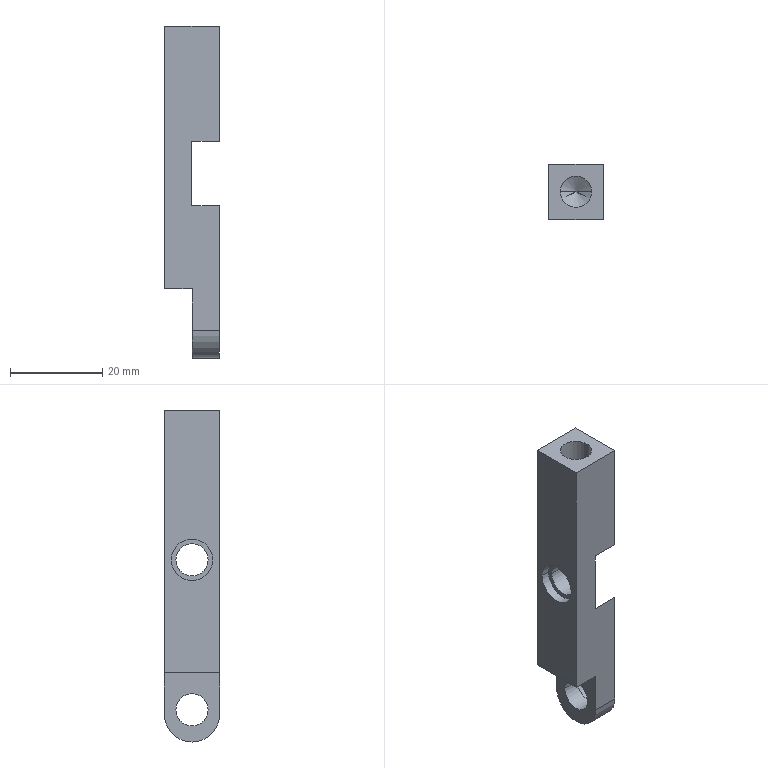Part | STEP file | Ngam kep 6 | 1 solid | 27 faces | box 11.9 x 12 x 72 mm | volume 6189 mm3 | plane 13 | cylinder 12 | cone 2 | commonest cylinder face diameters 7 x4 9 x4 6.8 x2 12 x2